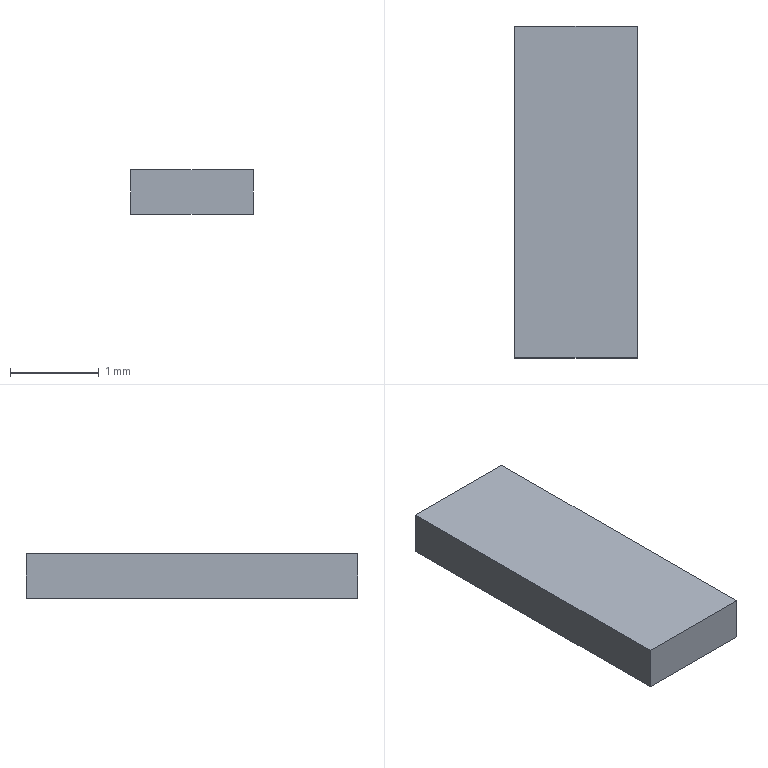Part | SolidWorks | features BaseBody 1 | 1 solid | 6 faces | box 1.375 x 3.74 x 0.5 mm | volume 2.572 mm3 | plane 6
STEP:
#1=CARTESIAN_POINT('',(-18.5,-12.25,2.5));
#2=VERTEX_POINT('',#1);
#3=CARTESIAN_POINT('',(-18.5,-15.99,2.5));
#4=VERTEX_POINT('',#3);
#5=CARTESIAN_POINT('',(-18.5,-12.25,2.5));
#6=DIRECTION('',(0.,-1.,0.));
#7=VECTOR('',#6,1000.);
#8=LINE('',#5,#7);
#9=EDGE_CURVE('',#2,#4,#8,.T.);
#10=ORIENTED_EDGE('',*,*,#9,.T.);
#11=CARTESIAN_POINT('',(-18.5,-15.99,3.));
#12=VERTEX_POINT('',#11);
#13=CARTESIAN_POINT('',(-18.5,-15.99,3.));
#14=DIRECTION('',(0.,0.,-1.));
#15=VECTOR('',#14,1000.);
#16=LINE('',#13,#15);
#17=EDGE_CURVE('',#12,#4,#16,.T.);
#18=ORIENTED_EDGE('',*,*,#17,.F.);
#19=CARTESIAN_POINT('',(-18.5,-12.25,3.));
#20=VERTEX_POINT('',#19);
#21=CARTESIAN_POINT('',(-18.5,-12.25,3.));
#22=DIRECTION('',(0.,-1.,0.));
#23=VECTOR('',#22,1000.);
#24=LINE('',#21,#23);
#25=EDGE_CURVE('',#20,#12,#24,.T.);
#26=ORIENTED_EDGE('',*,*,#25,.F.);
#27=CARTESIAN_POINT('',(-18.5,-12.25,3.));
#28=DIRECTION('',(0.,0.,-1.));
#29=VECTOR('',#28,1000.);
#30=LINE('',#27,#29);
#31=EDGE_CURVE('',#20,#2,#30,.T.);
#32=ORIENTED_EDGE('',*,*,#31,.T.);
#33=EDGE_LOOP('',(#10,#18,#26,#32));
#34=FACE_OUTER_BOUND('',#33,.T.);
#35=CARTESIAN_POINT('',(-18.5,-12.25,3.));
#36=DIRECTION('',(1.,0.,0.));
#37=DIRECTION('',(0.,0.,-1.));
#38=AXIS2_PLACEMENT_3D('',#35,#36,#37);
#39=PLANE('',#38);
#40=ADVANCED_FACE('',(#34),#39,.F.);
#41=CARTESIAN_POINT('',(-17.125,-15.99,2.5));
#42=VERTEX_POINT('',#41);
#43=CARTESIAN_POINT('',(-18.5,-15.99,2.5));
#44=DIRECTION('',(1.,0.,0.));
#45=VECTOR('',#44,1000.);
#46=LINE('',#43,#45);
#47=EDGE_CURVE('',#4,#42,#46,.T.);
#48=ORIENTED_EDGE('',*,*,#47,.T.);
#49=CARTESIAN_POINT('',(-17.125,-15.99,3.));
#50=VERTEX_POINT('',#49);
#51=CARTESIAN_POINT('',(-17.125,-15.99,3.));
#52=DIRECTION('',(0.,0.,-1.));
#53=VECTOR('',#52,1000.);
#54=LINE('',#51,#53);
#55=EDGE_CURVE('',#50,#42,#54,.T.);
#56=ORIENTED_EDGE('',*,*,#55,.F.);
#57=CARTESIAN_POINT('',(-18.5,-15.99,3.));
#58=DIRECTION('',(1.,0.,0.));
#59=VECTOR('',#58,1000.);
#60=LINE('',#57,#59);
#61=EDGE_CURVE('',#12,#50,#60,.T.);
#62=ORIENTED_EDGE('',*,*,#61,.F.);
#63=ORIENTED_EDGE('',*,*,#17,.T.);
#64=EDGE_LOOP('',(#48,#56,#62,#63));
#65=FACE_OUTER_BOUND('',#64,.T.);
#66=CARTESIAN_POINT('',(-18.5,-15.99,3.));
#67=DIRECTION('',(0.,1.,0.));
#68=DIRECTION('',(0.,0.,1.));
#69=AXIS2_PLACEMENT_3D('',#66,#67,#68);
#70=PLANE('',#69);
#71=ADVANCED_FACE('',(#65),#70,.F.);
#72=CARTESIAN_POINT('',(-17.125,-12.25,2.5));
#73=VERTEX_POINT('',#72);
#74=CARTESIAN_POINT('',(-17.125,-15.99,2.5));
#75=DIRECTION('',(0.,1.,0.));
#76=VECTOR('',#75,1000.);
#77=LINE('',#74,#76);
#78=EDGE_CURVE('',#42,#73,#77,.T.);
#79=ORIENTED_EDGE('',*,*,#78,.T.);
#80=CARTESIAN_POINT('',(-17.125,-12.25,3.));
#81=VERTEX_POINT('',#80);
#82=CARTESIAN_POINT('',(-17.125,-12.25,3.));
#83=DIRECTION('',(0.,0.,-1.));
#84=VECTOR('',#83,1000.);
#85=LINE('',#82,#84);
#86=EDGE_CURVE('',#81,#73,#85,.T.);
#87=ORIENTED_EDGE('',*,*,#86,.F.);
#88=CARTESIAN_POINT('',(-17.125,-15.99,3.));
#89=DIRECTION('',(0.,1.,0.));
#90=VECTOR('',#89,1000.);
#91=LINE('',#88,#90);
#92=EDGE_CURVE('',#50,#81,#91,.T.);
#93=ORIENTED_EDGE('',*,*,#92,.F.);
#94=ORIENTED_EDGE('',*,*,#55,.T.);
#95=EDGE_LOOP('',(#79,#87,#93,#94));
#96=FACE_OUTER_BOUND('',#95,.T.);
#97=CARTESIAN_POINT('',(-17.125,-15.99,3.));
#98=DIRECTION('',(-1.,0.,0.));
#99=DIRECTION('',(0.,0.,1.));
#100=AXIS2_PLACEMENT_3D('',#97,#98,#99);
#101=PLANE('',#100);
#102=ADVANCED_FACE('',(#96),#101,.F.);
#103=CARTESIAN_POINT('',(-17.125,-12.25,2.5));
#104=DIRECTION('',(-1.,0.,0.));
#105=VECTOR('',#104,1000.);
#106=LINE('',#103,#105);
#107=EDGE_CURVE('',#73,#2,#106,.T.);
#108=ORIENTED_EDGE('',*,*,#107,.T.);
#109=ORIENTED_EDGE('',*,*,#31,.F.);
#110=CARTESIAN_POINT('',(-17.125,-12.25,3.));
#111=DIRECTION('',(-1.,0.,0.));
#112=VECTOR('',#111,1000.);
#113=LINE('',#110,#112);
#114=EDGE_CURVE('',#81,#20,#113,.T.);
#115=ORIENTED_EDGE('',*,*,#114,.F.);
#116=ORIENTED_EDGE('',*,*,#86,.T.);
#117=EDGE_LOOP('',(#108,#109,#115,#116));
#118=FACE_OUTER_BOUND('',#117,.T.);
#119=CARTESIAN_POINT('',(-17.125,-12.25,3.));
#120=DIRECTION('',(0.,-1.,0.));
#121=DIRECTION('',(0.,0.,-1.));
#122=AXIS2_PLACEMENT_3D('',#119,#120,#121);
#123=PLANE('',#122);
#124=ADVANCED_FACE('',(#118),#123,.F.);
#125=ORIENTED_EDGE('',*,*,#25,.T.);
#126=ORIENTED_EDGE('',*,*,#61,.T.);
#127=ORIENTED_EDGE('',*,*,#92,.T.);
#128=ORIENTED_EDGE('',*,*,#114,.T.);
#129=EDGE_LOOP('',(#125,#126,#127,#128));
#130=FACE_OUTER_BOUND('',#129,.T.);
#131=CARTESIAN_POINT('',(0.,0.,3.));
#132=DIRECTION('',(0.,0.,1.));
#133=DIRECTION('',(1.,0.,0.));
#134=AXIS2_PLACEMENT_3D('',#131,#132,#133);
#135=PLANE('',#134);
#136=ADVANCED_FACE('',(#130),#135,.T.);
#137=ORIENTED_EDGE('',*,*,#9,.F.);
#138=ORIENTED_EDGE('',*,*,#107,.F.);
#139=ORIENTED_EDGE('',*,*,#78,.F.);
#140=ORIENTED_EDGE('',*,*,#47,.F.);
#141=EDGE_LOOP('',(#137,#138,#139,#140));
#142=FACE_OUTER_BOUND('',#141,.T.);
#143=CARTESIAN_POINT('',(0.,0.,2.5));
#144=DIRECTION('',(0.,0.,1.));
#145=DIRECTION('',(1.,0.,0.));
#146=AXIS2_PLACEMENT_3D('',#143,#144,#145);
#147=PLANE('',#146);
#148=ADVANCED_FACE('',(#142),#147,.F.);
#149=CLOSED_SHELL('',(#40,#71,#102,#124,#136,#148));
#150=MANIFOLD_SOLID_BREP('',#149);
#151=CARTESIAN_POINT('',(0.,0.,0.));
#152=DIRECTION('',(0.,0.,1.));
#153=DIRECTION('',(1.,0.,0.));
#154=AXIS2_PLACEMENT_3D('',#151,#152,#153);
#155=(LENGTH_UNIT()NAMED_UNIT(*)SI_UNIT(.MILLI.,.METRE.));
#156=UNCERTAINTY_MEASURE_WITH_UNIT(LENGTH_MEASURE(0.00001),#155,'','');
#157=(NAMED_UNIT(*)PLANE_ANGLE_UNIT()SI_UNIT($,.RADIAN.));
#158=(NAMED_UNIT(*)SI_UNIT($,.STERADIAN.)SOLID_ANGLE_UNIT());
#159=(GEOMETRIC_REPRESENTATION_CONTEXT(3)GLOBAL_UNCERTAINTY_ASSIGNED_CONTEXT((#156))GLOBAL_UNIT_ASSIGNED_CONTEXT((#155,#157,#158))REPRESENTATION_CONTEXT('',''));
#160=ADVANCED_BREP_SHAPE_REPRESENTATION('',(#150,#154),#159);